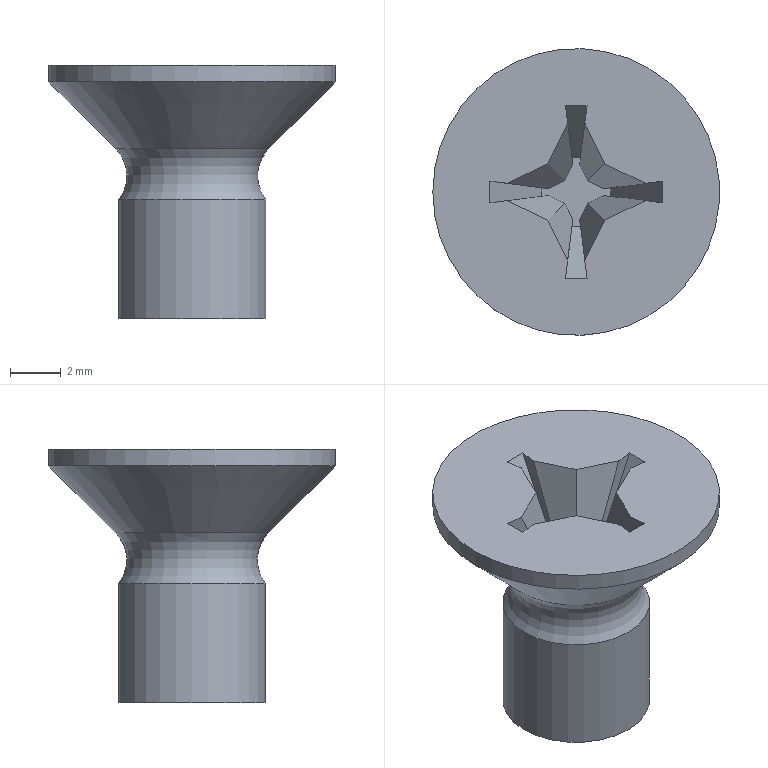Part | NX | features SKETCH 3, DATUM_CSYS 2, DATUM_PLANE 1, FSET 1, LINE 1, META 1, SKIN 1, SWP104 1, SYMBOLIC_THREAD 1, THREADS 1 | 1 solid | 27 faces | box 11.3 x 11.3 x 10 mm | volume 366.572 mm3 | plane 23 | cylinder 2 | torus 1 | cone 1 | commonest cylinder face diameters 5.795 x1 11.3 x1
STEP:
#1=CARTESIAN_POINT('',(-2.897,0.,-5.3));
#2=VERTEX_POINT('',#1);
#3=CARTESIAN_POINT('',(0.,0.,-5.3));
#4=DIRECTION('',(0.,0.,-1.));
#5=DIRECTION('',(-1.,0.,0.));
#6=AXIS2_PLACEMENT_3D('',#3,#4,#5);
#7=CIRCLE('',#6,2.897);
#8=EDGE_CURVE('',#2,#2,#7,.T.);
#9=ORIENTED_EDGE('',*,*,#8,.F.);
#10=EDGE_LOOP('',(#9));
#11=FACE_BOUND('',#10,.T.);
#12=CARTESIAN_POINT('',(-3.014,0.,-3.3));
#13=VERTEX_POINT('',#12);
#14=CARTESIAN_POINT('',(0.,0.,-3.3));
#15=DIRECTION('',(0.,0.,-1.));
#16=DIRECTION('',(-1.,0.,0.));
#17=AXIS2_PLACEMENT_3D('',#14,#15,#16);
#18=CIRCLE('',#17,3.014);
#19=EDGE_CURVE('',#13,#13,#18,.T.);
#20=ORIENTED_EDGE('',*,*,#19,.T.);
#21=EDGE_LOOP('',(#20));
#22=FACE_BOUND('',#21,.T.);
#23=CARTESIAN_POINT('',(0.,0.,-4.366));
#24=DIRECTION('',(0.,0.,-1.));
#25=DIRECTION('',(-1.,0.,0.));
#26=AXIS2_PLACEMENT_3D('',#23,#24,#25);
#27=TOROIDAL_SURFACE('',#26,4.08,1.507);
#28=ADVANCED_FACE('',(#11,#22),#27,.F.);
#29=CARTESIAN_POINT('',(-2.898,0.,-10.));
#30=VERTEX_POINT('',#29);
#31=CARTESIAN_POINT('',(0.,0.,-10.));
#32=DIRECTION('',(0.,0.,-1.));
#33=DIRECTION('',(-1.,0.,0.));
#34=AXIS2_PLACEMENT_3D('',#31,#32,#33);
#35=CIRCLE('',#34,2.898);
#36=EDGE_CURVE('',#30,#30,#35,.T.);
#37=ORIENTED_EDGE('',*,*,#36,.F.);
#38=EDGE_LOOP('',(#37));
#39=FACE_BOUND('',#38,.T.);
#40=ORIENTED_EDGE('',*,*,#8,.T.);
#41=EDGE_LOOP('',(#40));
#42=FACE_BOUND('',#41,.T.);
#43=CARTESIAN_POINT('',(0.,0.,0.));
#44=DIRECTION('',(0.,0.,-1.));
#45=DIRECTION('',(-1.,0.,0.));
#46=AXIS2_PLACEMENT_3D('',#43,#44,#45);
#47=CYLINDRICAL_SURFACE('',#46,2.898);
#48=ADVANCED_FACE('',(#39,#42),#47,.T.);
#49=ORIENTED_EDGE('',*,*,#36,.T.);
#50=EDGE_LOOP('',(#49));
#51=FACE_BOUND('',#50,.T.);
#52=CARTESIAN_POINT('',(0.,2.898,-10.));
#53=DIRECTION('',(0.,0.,1.));
#54=DIRECTION('',(1.,0.,0.));
#55=AXIS2_PLACEMENT_3D('',#52,#53,#54);
#56=PLANE('',#55);
#57=ADVANCED_FACE('',(#51),#56,.F.);
#58=CARTESIAN_POINT('',(3.4,-0.425,0.));
#59=VERTEX_POINT('',#58);
#60=CARTESIAN_POINT('',(2.72,-0.34,0.));
#61=VERTEX_POINT('',#60);
#62=CARTESIAN_POINT('',(3.06,-0.3825,0.));
#63=DIRECTION('',(-0.9923,0.124,0.));
#64=VECTOR('',#63,1000.);
#65=LINE('',#62,#64);
#66=EDGE_CURVE('',#59,#61,#65,.T.);
#67=ORIENTED_EDGE('',*,*,#66,.T.);
#68=CARTESIAN_POINT('',(1.117,-1.117,0.));
#69=VERTEX_POINT('',#68);
#70=CARTESIAN_POINT('',(1.919,-0.7287,0.));
#71=DIRECTION('',(-0.8997,-0.4364,0.));
#72=VECTOR('',#71,1000.);
#73=LINE('',#70,#72);
#74=EDGE_CURVE('',#61,#69,#73,.T.);
#75=ORIENTED_EDGE('',*,*,#74,.T.);
#76=CARTESIAN_POINT('',(0.34,-2.72,0.));
#77=VERTEX_POINT('',#76);
#78=CARTESIAN_POINT('',(0.7287,-1.919,0.));
#79=DIRECTION('',(-0.4364,-0.8997,0.));
#80=VECTOR('',#79,1000.);
#81=LINE('',#78,#80);
#82=EDGE_CURVE('',#69,#77,#81,.T.);
#83=ORIENTED_EDGE('',*,*,#82,.T.);
#84=CARTESIAN_POINT('',(0.425,-3.4,0.));
#85=VERTEX_POINT('',#84);
#86=CARTESIAN_POINT('',(0.3825,-3.06,0.));
#87=DIRECTION('',(0.124,-0.9923,0.));
#88=VECTOR('',#87,1000.);
#89=LINE('',#86,#88);
#90=EDGE_CURVE('',#77,#85,#89,.T.);
#91=ORIENTED_EDGE('',*,*,#90,.T.);
#92=CARTESIAN_POINT('',(-0.425,-3.4,0.));
#93=VERTEX_POINT('',#92);
#94=CARTESIAN_POINT('',(0.2125,-3.4,0.));
#95=DIRECTION('',(-1.,0.,0.));
#96=VECTOR('',#95,1000.);
#97=LINE('',#94,#96);
#98=EDGE_CURVE('',#85,#93,#97,.T.);
#99=ORIENTED_EDGE('',*,*,#98,.T.);
#100=CARTESIAN_POINT('',(-0.34,-2.72,0.));
#101=VERTEX_POINT('',#100);
#102=CARTESIAN_POINT('',(-0.3825,-3.06,0.));
#103=DIRECTION('',(0.124,0.9923,0.));
#104=VECTOR('',#103,1000.);
#105=LINE('',#102,#104);
#106=EDGE_CURVE('',#93,#101,#105,.T.);
#107=ORIENTED_EDGE('',*,*,#106,.T.);
#108=CARTESIAN_POINT('',(-1.117,-1.117,0.));
#109=VERTEX_POINT('',#108);
#110=CARTESIAN_POINT('',(-0.7287,-1.919,0.));
#111=DIRECTION('',(-0.4364,0.8997,0.));
#112=VECTOR('',#111,1000.);
#113=LINE('',#110,#112);
#114=EDGE_CURVE('',#101,#109,#113,.T.);
#115=ORIENTED_EDGE('',*,*,#114,.T.);
#116=CARTESIAN_POINT('',(-2.72,-0.34,0.));
#117=VERTEX_POINT('',#116);
#118=CARTESIAN_POINT('',(-1.919,-0.7287,0.));
#119=DIRECTION('',(-0.8997,0.4364,0.));
#120=VECTOR('',#119,1000.);
#121=LINE('',#118,#120);
#122=EDGE_CURVE('',#109,#117,#121,.T.);
#123=ORIENTED_EDGE('',*,*,#122,.T.);
#124=CARTESIAN_POINT('',(-3.4,-0.425,0.));
#125=VERTEX_POINT('',#124);
#126=CARTESIAN_POINT('',(-3.06,-0.3825,0.));
#127=DIRECTION('',(-0.9923,-0.124,0.));
#128=VECTOR('',#127,1000.);
#129=LINE('',#126,#128);
#130=EDGE_CURVE('',#117,#125,#129,.T.);
#131=ORIENTED_EDGE('',*,*,#130,.T.);
#132=CARTESIAN_POINT('',(-3.4,0.425,0.));
#133=VERTEX_POINT('',#132);
#134=CARTESIAN_POINT('',(-3.4,-0.2125,0.));
#135=DIRECTION('',(0.,1.,0.));
#136=VECTOR('',#135,1000.);
#137=LINE('',#134,#136);
#138=EDGE_CURVE('',#125,#133,#137,.T.);
#139=ORIENTED_EDGE('',*,*,#138,.T.);
#140=CARTESIAN_POINT('',(-2.72,0.34,0.));
#141=VERTEX_POINT('',#140);
#142=CARTESIAN_POINT('',(-3.06,0.3825,0.));
#143=DIRECTION('',(0.9923,-0.124,0.));
#144=VECTOR('',#143,1000.);
#145=LINE('',#142,#144);
#146=EDGE_CURVE('',#133,#141,#145,.T.);
#147=ORIENTED_EDGE('',*,*,#146,.T.);
#148=CARTESIAN_POINT('',(-1.117,1.117,0.));
#149=VERTEX_POINT('',#148);
#150=CARTESIAN_POINT('',(-1.919,0.7287,0.));
#151=DIRECTION('',(0.8997,0.4364,0.));
#152=VECTOR('',#151,1000.);
#153=LINE('',#150,#152);
#154=EDGE_CURVE('',#141,#149,#153,.T.);
#155=ORIENTED_EDGE('',*,*,#154,.T.);
#156=CARTESIAN_POINT('',(-0.34,2.72,0.));
#157=VERTEX_POINT('',#156);
#158=CARTESIAN_POINT('',(-0.7287,1.919,0.));
#159=DIRECTION('',(0.4364,0.8997,0.));
#160=VECTOR('',#159,1000.);
#161=LINE('',#158,#160);
#162=EDGE_CURVE('',#149,#157,#161,.T.);
#163=ORIENTED_EDGE('',*,*,#162,.T.);
#164=CARTESIAN_POINT('',(-0.425,3.4,0.));
#165=VERTEX_POINT('',#164);
#166=CARTESIAN_POINT('',(-0.3825,3.06,0.));
#167=DIRECTION('',(-0.124,0.9923,0.));
#168=VECTOR('',#167,1000.);
#169=LINE('',#166,#168);
#170=EDGE_CURVE('',#157,#165,#169,.T.);
#171=ORIENTED_EDGE('',*,*,#170,.T.);
#172=CARTESIAN_POINT('',(0.425,3.4,0.));
#173=VERTEX_POINT('',#172);
#174=CARTESIAN_POINT('',(-0.2125,3.4,0.));
#175=DIRECTION('',(1.,0.,0.));
#176=VECTOR('',#175,1000.);
#177=LINE('',#174,#176);
#178=EDGE_CURVE('',#165,#173,#177,.T.);
#179=ORIENTED_EDGE('',*,*,#178,.T.);
#180=CARTESIAN_POINT('',(0.34,2.72,0.));
#181=VERTEX_POINT('',#180);
#182=CARTESIAN_POINT('',(0.3825,3.06,0.));
#183=DIRECTION('',(-0.124,-0.9923,0.));
#184=VECTOR('',#183,1000.);
#185=LINE('',#182,#184);
#186=EDGE_CURVE('',#173,#181,#185,.T.);
#187=ORIENTED_EDGE('',*,*,#186,.T.);
#188=CARTESIAN_POINT('',(1.117,1.117,0.));
#189=VERTEX_POINT('',#188);
#190=CARTESIAN_POINT('',(0.7287,1.919,0.));
#191=DIRECTION('',(0.4364,-0.8997,0.));
#192=VECTOR('',#191,1000.);
#193=LINE('',#190,#192);
#194=EDGE_CURVE('',#181,#189,#193,.T.);
#195=ORIENTED_EDGE('',*,*,#194,.T.);
#196=CARTESIAN_POINT('',(2.72,0.34,0.));
#197=VERTEX_POINT('',#196);
#198=CARTESIAN_POINT('',(1.919,0.7287,0.));
#199=DIRECTION('',(0.8997,-0.4364,0.));
#200=VECTOR('',#199,1000.);
#201=LINE('',#198,#200);
#202=EDGE_CURVE('',#189,#197,#201,.T.);
#203=ORIENTED_EDGE('',*,*,#202,.T.);
#204=CARTESIAN_POINT('',(3.4,0.425,0.));
#205=VERTEX_POINT('',#204);
#206=CARTESIAN_POINT('',(3.06,0.3825,0.));
#207=DIRECTION('',(0.9923,0.124,0.));
#208=VECTOR('',#207,1000.);
#209=LINE('',#206,#208);
#210=EDGE_CURVE('',#197,#205,#209,.T.);
#211=ORIENTED_EDGE('',*,*,#210,.T.);
#212=CARTESIAN_POINT('',(3.4,0.2125,0.));
#213=DIRECTION('',(0.,-1.,0.));
#214=VECTOR('',#213,1000.);
#215=LINE('',#212,#214);
#216=EDGE_CURVE('',#205,#59,#215,.T.);
#217=ORIENTED_EDGE('',*,*,#216,.T.);
#218=EDGE_LOOP('',(#67,#75,#83,#91,#99,#107,#115,#123,#131,#139,#147,#155,#163,#171,#179,#187,#195,#203,#211,#217));
#219=FACE_BOUND('',#218,.T.);
#220=CARTESIAN_POINT('',(-5.65,0.,0.));
#221=VERTEX_POINT('',#220);
#222=CARTESIAN_POINT('',(0.,0.,0.));
#223=DIRECTION('',(0.,0.,-1.));
#224=DIRECTION('',(-1.,0.,0.));
#225=AXIS2_PLACEMENT_3D('',#222,#223,#224);
#226=CIRCLE('',#225,5.65);
#227=EDGE_CURVE('',#221,#221,#226,.T.);
#228=ORIENTED_EDGE('',*,*,#227,.F.);
#229=EDGE_LOOP('',(#228));
#230=FACE_BOUND('',#229,.T.);
#231=CARTESIAN_POINT('',(0.,0.,0.));
#232=DIRECTION('',(0.,0.,-1.));
#233=DIRECTION('',(-1.,0.,0.));
#234=AXIS2_PLACEMENT_3D('',#231,#232,#233);
#235=PLANE('',#234);
#236=ADVANCED_FACE('',(#219,#230),#235,.F.);
#237=CARTESIAN_POINT('',(-5.65,0.,-0.6641));
#238=VERTEX_POINT('',#237);
#239=CARTESIAN_POINT('',(0.,0.,-0.6641));
#240=DIRECTION('',(0.,0.,-1.));
#241=DIRECTION('',(-1.,0.,0.));
#242=AXIS2_PLACEMENT_3D('',#239,#240,#241);
#243=CIRCLE('',#242,5.65);
#244=EDGE_CURVE('',#238,#238,#243,.T.);
#245=ORIENTED_EDGE('',*,*,#244,.F.);
#246=EDGE_LOOP('',(#245));
#247=FACE_BOUND('',#246,.T.);
#248=ORIENTED_EDGE('',*,*,#227,.T.);
#249=EDGE_LOOP('',(#248));
#250=FACE_BOUND('',#249,.T.);
#251=CARTESIAN_POINT('',(0.,0.,0.));
#252=DIRECTION('',(0.,0.,-1.));
#253=DIRECTION('',(-1.,0.,0.));
#254=AXIS2_PLACEMENT_3D('',#251,#252,#253);
#255=CYLINDRICAL_SURFACE('',#254,5.65);
#256=ADVANCED_FACE('',(#247,#250),#255,.T.);
#257=ORIENTED_EDGE('',*,*,#19,.F.);
#258=EDGE_LOOP('',(#257));
#259=FACE_BOUND('',#258,.T.);
#260=ORIENTED_EDGE('',*,*,#244,.T.);
#261=EDGE_LOOP('',(#260));
#262=FACE_BOUND('',#261,.T.);
#263=CARTESIAN_POINT('',(0.,0.,-0.6641));
#264=DIRECTION('',(0.,0.,1.));
#265=DIRECTION('',(1.,0.,0.));
#266=AXIS2_PLACEMENT_3D('',#263,#264,#265);
#267=CONICAL_SURFACE('',#266,5.65,0.7854);
#268=ADVANCED_FACE('',(#259,#262),#267,.T.);
#269=CARTESIAN_POINT('',(1.36,-0.17,-3.5));
#270=VERTEX_POINT('',#269);
#271=CARTESIAN_POINT('',(2.38,-0.2975,-1.75));
#272=DIRECTION('',(0.5026,-0.06282,0.8623));
#273=VECTOR('',#272,1000.);
#274=LINE('',#271,#273);
#275=EDGE_CURVE('',#270,#59,#274,.T.);
#276=ORIENTED_EDGE('',*,*,#275,.F.);
#277=CARTESIAN_POINT('',(1.088,-0.136,-3.5));
#278=VERTEX_POINT('',#277);
#279=CARTESIAN_POINT('',(1.224,-0.153,-3.5));
#280=DIRECTION('',(-0.9923,0.124,0.));
#281=VECTOR('',#280,1000.);
#282=LINE('',#279,#281);
#283=EDGE_CURVE('',#270,#278,#282,.T.);
#284=ORIENTED_EDGE('',*,*,#283,.T.);
#285=CARTESIAN_POINT('',(1.904,-0.238,-1.75));
#286=DIRECTION('',(0.422,-0.05275,0.9051));
#287=VECTOR('',#286,1000.);
#288=LINE('',#285,#287);
#289=EDGE_CURVE('',#278,#61,#288,.T.);
#290=ORIENTED_EDGE('',*,*,#289,.T.);
#291=ORIENTED_EDGE('',*,*,#66,.F.);
#292=EDGE_LOOP('',(#276,#284,#290,#291));
#293=FACE_BOUND('',#292,.T.);
#294=CARTESIAN_POINT('',(2.38,-0.2975,-1.75));
#295=DIRECTION('',(0.124,0.9923,0.));
#296=DIRECTION('',(-0.9923,0.124,0.));
#297=AXIS2_PLACEMENT_3D('',#294,#295,#296);
#298=PLANE('',#297);
#299=ADVANCED_FACE('',(#293),#298,.T.);
#300=CARTESIAN_POINT('',(1.36,0.17,-3.5));
#301=VERTEX_POINT('',#300);
#302=CARTESIAN_POINT('',(2.38,0.2975,-1.75));
#303=DIRECTION('',(0.5026,0.06282,0.8623));
#304=VECTOR('',#303,1000.);
#305=LINE('',#302,#304);
#306=EDGE_CURVE('',#301,#205,#305,.T.);
#307=ORIENTED_EDGE('',*,*,#306,.F.);
#308=CARTESIAN_POINT('',(1.36,0.085,-3.5));
#309=DIRECTION('',(0.,-1.,0.));
#310=VECTOR('',#309,1000.);
#311=LINE('',#308,#310);
#312=EDGE_CURVE('',#301,#270,#311,.T.);
#313=ORIENTED_EDGE('',*,*,#312,.T.);
#314=ORIENTED_EDGE('',*,*,#275,.T.);
#315=ORIENTED_EDGE('',*,*,#216,.F.);
#316=EDGE_LOOP('',(#307,#313,#314,#315));
#317=FACE_BOUND('',#316,.T.);
#318=CARTESIAN_POINT('',(2.38,0.2975,-1.75));
#319=DIRECTION('',(-0.864,0.,0.5036));
#320=DIRECTION('',(0.5036,0.,0.864));
#321=AXIS2_PLACEMENT_3D('',#318,#319,#320);
#322=PLANE('',#321);
#323=ADVANCED_FACE('',(#317),#322,.T.);
#324=CARTESIAN_POINT('',(1.088,0.136,-3.5));
#325=VERTEX_POINT('',#324);
#326=CARTESIAN_POINT('',(1.904,0.238,-1.75));
#327=DIRECTION('',(0.422,0.05275,0.9051));
#328=VECTOR('',#327,1000.);
#329=LINE('',#326,#328);
#330=EDGE_CURVE('',#325,#197,#329,.T.);
#331=ORIENTED_EDGE('',*,*,#330,.F.);
#332=CARTESIAN_POINT('',(1.224,0.153,-3.5));
#333=DIRECTION('',(0.9923,0.124,0.));
#334=VECTOR('',#333,1000.);
#335=LINE('',#332,#334);
#336=EDGE_CURVE('',#325,#301,#335,.T.);
#337=ORIENTED_EDGE('',*,*,#336,.T.);
#338=ORIENTED_EDGE('',*,*,#306,.T.);
#339=ORIENTED_EDGE('',*,*,#210,.F.);
#340=EDGE_LOOP('',(#331,#337,#338,#339));
#341=FACE_BOUND('',#340,.T.);
#342=CARTESIAN_POINT('',(2.38,0.2975,-1.75));
#343=DIRECTION('',(0.124,-0.9923,0.));
#344=DIRECTION('',(0.9923,0.124,0.));
#345=AXIS2_PLACEMENT_3D('',#342,#343,#344);
#346=PLANE('',#345);
#347=ADVANCED_FACE('',(#341),#346,.T.);
#348=CARTESIAN_POINT('',(0.4469,0.4469,-3.5));
#349=VERTEX_POINT('',#348);
#350=CARTESIAN_POINT('',(0.7821,0.7821,-1.75));
#351=DIRECTION('',(0.1849,0.1849,0.9652));
#352=VECTOR('',#351,1000.);
#353=LINE('',#350,#352);
#354=EDGE_CURVE('',#349,#189,#353,.T.);
#355=ORIENTED_EDGE('',*,*,#354,.F.);
#356=CARTESIAN_POINT('',(0.7675,0.2915,-3.5));
#357=DIRECTION('',(0.8997,-0.4364,0.));
#358=VECTOR('',#357,1000.);
#359=LINE('',#356,#358);
#360=EDGE_CURVE('',#349,#325,#359,.T.);
#361=ORIENTED_EDGE('',*,*,#360,.T.);
#362=ORIENTED_EDGE('',*,*,#330,.T.);
#363=ORIENTED_EDGE('',*,*,#202,.F.);
#364=EDGE_LOOP('',(#355,#361,#362,#363));
#365=FACE_BOUND('',#364,.T.);
#366=CARTESIAN_POINT('',(1.904,0.238,-1.75));
#367=DIRECTION('',(-0.4228,-0.8717,0.2479));
#368=DIRECTION('',(0.8997,-0.4364,0.));
#369=AXIS2_PLACEMENT_3D('',#366,#367,#368);
#370=PLANE('',#369);
#371=ADVANCED_FACE('',(#365),#370,.T.);
#372=CARTESIAN_POINT('',(0.136,1.088,-3.5));
#373=VERTEX_POINT('',#372);
#374=CARTESIAN_POINT('',(0.238,1.904,-1.75));
#375=DIRECTION('',(0.05275,0.422,0.9051));
#376=VECTOR('',#375,1000.);
#377=LINE('',#374,#376);
#378=EDGE_CURVE('',#373,#181,#377,.T.);
#379=ORIENTED_EDGE('',*,*,#378,.F.);
#380=CARTESIAN_POINT('',(0.2915,0.7675,-3.5));
#381=DIRECTION('',(0.4364,-0.8997,0.));
#382=VECTOR('',#381,1000.);
#383=LINE('',#380,#382);
#384=EDGE_CURVE('',#373,#349,#383,.T.);
#385=ORIENTED_EDGE('',*,*,#384,.T.);
#386=ORIENTED_EDGE('',*,*,#354,.T.);
#387=ORIENTED_EDGE('',*,*,#194,.F.);
#388=EDGE_LOOP('',(#379,#385,#386,#387));
#389=FACE_BOUND('',#388,.T.);
#390=CARTESIAN_POINT('',(0.238,1.904,-1.75));
#391=DIRECTION('',(-0.8717,-0.4228,0.2479));
#392=DIRECTION('',(0.4364,-0.8997,0.));
#393=AXIS2_PLACEMENT_3D('',#390,#391,#392);
#394=PLANE('',#393);
#395=ADVANCED_FACE('',(#389),#394,.T.);
#396=CARTESIAN_POINT('',(0.17,1.36,-3.5));
#397=VERTEX_POINT('',#396);
#398=CARTESIAN_POINT('',(0.2975,2.38,-1.75));
#399=DIRECTION('',(0.06282,0.5026,0.8623));
#400=VECTOR('',#399,1000.);
#401=LINE('',#398,#400);
#402=EDGE_CURVE('',#397,#173,#401,.T.);
#403=ORIENTED_EDGE('',*,*,#402,.F.);
#404=CARTESIAN_POINT('',(0.153,1.224,-3.5));
#405=DIRECTION('',(-0.124,-0.9923,0.));
#406=VECTOR('',#405,1000.);
#407=LINE('',#404,#406);
#408=EDGE_CURVE('',#397,#373,#407,.T.);
#409=ORIENTED_EDGE('',*,*,#408,.T.);
#410=ORIENTED_EDGE('',*,*,#378,.T.);
#411=ORIENTED_EDGE('',*,*,#186,.F.);
#412=EDGE_LOOP('',(#403,#409,#410,#411));
#413=FACE_BOUND('',#412,.T.);
#414=CARTESIAN_POINT('',(0.2975,2.38,-1.75));
#415=DIRECTION('',(-0.9923,0.124,0.));
#416=DIRECTION('',(-0.124,-0.9923,0.));
#417=AXIS2_PLACEMENT_3D('',#414,#415,#416);
#418=PLANE('',#417);
#419=ADVANCED_FACE('',(#413),#418,.T.);
#420=CARTESIAN_POINT('',(-0.17,1.36,-3.5));
#421=VERTEX_POINT('',#420);
#422=CARTESIAN_POINT('',(-0.2975,2.38,-1.75));
#423=DIRECTION('',(-0.06282,0.5026,0.8623));
#424=VECTOR('',#423,1000.);
#425=LINE('',#422,#424);
#426=EDGE_CURVE('',#421,#165,#425,.T.);
#427=ORIENTED_EDGE('',*,*,#426,.F.);
#428=CARTESIAN_POINT('',(-0.085,1.36,-3.5));
#429=DIRECTION('',(1.,0.,0.));
#430=VECTOR('',#429,1000.);
#431=LINE('',#428,#430);
#432=EDGE_CURVE('',#421,#397,#431,.T.);
#433=ORIENTED_EDGE('',*,*,#432,.T.);
#434=ORIENTED_EDGE('',*,*,#402,.T.);
#435=ORIENTED_EDGE('',*,*,#178,.F.);
#436=EDGE_LOOP('',(#427,#433,#434,#435));
#437=FACE_BOUND('',#436,.T.);
#438=CARTESIAN_POINT('',(-0.2975,2.38,-1.75));
#439=DIRECTION('',(0.,-0.864,0.5036));
#440=DIRECTION('',(0.,-0.5036,-0.864));
#441=AXIS2_PLACEMENT_3D('',#438,#439,#440);
#442=PLANE('',#441);
#443=ADVANCED_FACE('',(#437),#442,.T.);
#444=CARTESIAN_POINT('',(-0.136,1.088,-3.5));
#445=VERTEX_POINT('',#444);
#446=CARTESIAN_POINT('',(-0.238,1.904,-1.75));
#447=DIRECTION('',(-0.05275,0.422,0.9051));
#448=VECTOR('',#447,1000.);
#449=LINE('',#446,#448);
#450=EDGE_CURVE('',#445,#157,#449,.T.);
#451=ORIENTED_EDGE('',*,*,#450,.F.);
#452=CARTESIAN_POINT('',(-0.153,1.224,-3.5));
#453=DIRECTION('',(-0.124,0.9923,0.));
#454=VECTOR('',#453,1000.);
#455=LINE('',#452,#454);
#456=EDGE_CURVE('',#445,#421,#455,.T.);
#457=ORIENTED_EDGE('',*,*,#456,.T.);
#458=ORIENTED_EDGE('',*,*,#426,.T.);
#459=ORIENTED_EDGE('',*,*,#170,.F.);
#460=EDGE_LOOP('',(#451,#457,#458,#459));
#461=FACE_BOUND('',#460,.T.);
#462=CARTESIAN_POINT('',(-0.2975,2.38,-1.75));
#463=DIRECTION('',(0.9923,0.124,0.));
#464=DIRECTION('',(-0.124,0.9923,0.));
#465=AXIS2_PLACEMENT_3D('',#462,#463,#464);
#466=PLANE('',#465);
#467=ADVANCED_FACE('',(#461),#466,.T.);
#468=CARTESIAN_POINT('',(-0.4469,0.4469,-3.5));
#469=VERTEX_POINT('',#468);
#470=CARTESIAN_POINT('',(-0.7821,0.7821,-1.75));
#471=DIRECTION('',(-0.1849,0.1849,0.9652));
#472=VECTOR('',#471,1000.);
#473=LINE('',#470,#472);
#474=EDGE_CURVE('',#469,#149,#473,.T.);
#475=ORIENTED_EDGE('',*,*,#474,.F.);
#476=CARTESIAN_POINT('',(-0.2915,0.7675,-3.5));
#477=DIRECTION('',(0.4364,0.8997,0.));
#478=VECTOR('',#477,1000.);
#479=LINE('',#476,#478);
#480=EDGE_CURVE('',#469,#445,#479,.T.);
#481=ORIENTED_EDGE('',*,*,#480,.T.);
#482=ORIENTED_EDGE('',*,*,#450,.T.);
#483=ORIENTED_EDGE('',*,*,#162,.F.);
#484=EDGE_LOOP('',(#475,#481,#482,#483));
#485=FACE_BOUND('',#484,.T.);
#486=CARTESIAN_POINT('',(-0.238,1.904,-1.75));
#487=DIRECTION('',(0.8717,-0.4228,0.2479));
#488=DIRECTION('',(0.4364,0.8997,0.));
#489=AXIS2_PLACEMENT_3D('',#486,#487,#488);
#490=PLANE('',#489);
#491=ADVANCED_FACE('',(#485),#490,.T.);
#492=CARTESIAN_POINT('',(-1.088,0.136,-3.5));
#493=VERTEX_POINT('',#492);
#494=CARTESIAN_POINT('',(-1.904,0.238,-1.75));
#495=DIRECTION('',(-0.422,0.05275,0.9051));
#496=VECTOR('',#495,1000.);
#497=LINE('',#494,#496);
#498=EDGE_CURVE('',#493,#141,#497,.T.);
#499=ORIENTED_EDGE('',*,*,#498,.F.);
#500=CARTESIAN_POINT('',(-0.7675,0.2915,-3.5));
#501=DIRECTION('',(0.8997,0.4364,0.));
#502=VECTOR('',#501,1000.);
#503=LINE('',#500,#502);
#504=EDGE_CURVE('',#493,#469,#503,.T.);
#505=ORIENTED_EDGE('',*,*,#504,.T.);
#506=ORIENTED_EDGE('',*,*,#474,.T.);
#507=ORIENTED_EDGE('',*,*,#154,.F.);
#508=EDGE_LOOP('',(#499,#505,#506,#507));
#509=FACE_BOUND('',#508,.T.);
#510=CARTESIAN_POINT('',(-1.904,0.238,-1.75));
#511=DIRECTION('',(0.4228,-0.8717,0.2479));
#512=DIRECTION('',(0.8997,0.4364,0.));
#513=AXIS2_PLACEMENT_3D('',#510,#511,#512);
#514=PLANE('',#513);
#515=ADVANCED_FACE('',(#509),#514,.T.);
#516=CARTESIAN_POINT('',(-1.36,0.17,-3.5));
#517=VERTEX_POINT('',#516);
#518=CARTESIAN_POINT('',(-2.38,0.2975,-1.75));
#519=DIRECTION('',(-0.5026,0.06282,0.8623));
#520=VECTOR('',#519,1000.);
#521=LINE('',#518,#520);
#522=EDGE_CURVE('',#517,#133,#521,.T.);
#523=ORIENTED_EDGE('',*,*,#522,.F.);
#524=CARTESIAN_POINT('',(-1.224,0.153,-3.5));
#525=DIRECTION('',(0.9923,-0.124,0.));
#526=VECTOR('',#525,1000.);
#527=LINE('',#524,#526);
#528=EDGE_CURVE('',#517,#493,#527,.T.);
#529=ORIENTED_EDGE('',*,*,#528,.T.);
#530=ORIENTED_EDGE('',*,*,#498,.T.);
#531=ORIENTED_EDGE('',*,*,#146,.F.);
#532=EDGE_LOOP('',(#523,#529,#530,#531));
#533=FACE_BOUND('',#532,.T.);
#534=CARTESIAN_POINT('',(-2.38,0.2975,-1.75));
#535=DIRECTION('',(-0.124,-0.9923,0.));
#536=DIRECTION('',(0.9923,-0.124,0.));
#537=AXIS2_PLACEMENT_3D('',#534,#535,#536);
#538=PLANE('',#537);
#539=ADVANCED_FACE('',(#533),#538,.T.);
#540=CARTESIAN_POINT('',(-1.36,-0.17,-3.5));
#541=VERTEX_POINT('',#540);
#542=CARTESIAN_POINT('',(-2.38,-0.2975,-1.75));
#543=DIRECTION('',(-0.5026,-0.06282,0.8623));
#544=VECTOR('',#543,1000.);
#545=LINE('',#542,#544);
#546=EDGE_CURVE('',#541,#125,#545,.T.);
#547=ORIENTED_EDGE('',*,*,#546,.F.);
#548=CARTESIAN_POINT('',(-1.36,-0.085,-3.5));
#549=DIRECTION('',(0.,1.,0.));
#550=VECTOR('',#549,1000.);
#551=LINE('',#548,#550);
#552=EDGE_CURVE('',#541,#517,#551,.T.);
#553=ORIENTED_EDGE('',*,*,#552,.T.);
#554=ORIENTED_EDGE('',*,*,#522,.T.);
#555=ORIENTED_EDGE('',*,*,#138,.F.);
#556=EDGE_LOOP('',(#547,#553,#554,#555));
#557=FACE_BOUND('',#556,.T.);
#558=CARTESIAN_POINT('',(-2.38,-0.2975,-1.75));
#559=DIRECTION('',(0.864,0.,0.5036));
#560=DIRECTION('',(0.5036,0.,-0.864));
#561=AXIS2_PLACEMENT_3D('',#558,#559,#560);
#562=PLANE('',#561);
#563=ADVANCED_FACE('',(#557),#562,.T.);
#564=CARTESIAN_POINT('',(-1.088,-0.136,-3.5));
#565=VERTEX_POINT('',#564);
#566=CARTESIAN_POINT('',(-1.904,-0.238,-1.75));
#567=DIRECTION('',(-0.422,-0.05275,0.9051));
#568=VECTOR('',#567,1000.);
#569=LINE('',#566,#568);
#570=EDGE_CURVE('',#565,#117,#569,.T.);
#571=ORIENTED_EDGE('',*,*,#570,.F.);
#572=CARTESIAN_POINT('',(-1.224,-0.153,-3.5));
#573=DIRECTION('',(-0.9923,-0.124,0.));
#574=VECTOR('',#573,1000.);
#575=LINE('',#572,#574);
#576=EDGE_CURVE('',#565,#541,#575,.T.);
#577=ORIENTED_EDGE('',*,*,#576,.T.);
#578=ORIENTED_EDGE('',*,*,#546,.T.);
#579=ORIENTED_EDGE('',*,*,#130,.F.);
#580=EDGE_LOOP('',(#571,#577,#578,#579));
#581=FACE_BOUND('',#580,.T.);
#582=CARTESIAN_POINT('',(-2.38,-0.2975,-1.75));
#583=DIRECTION('',(-0.124,0.9923,0.));
#584=DIRECTION('',(-0.9923,-0.124,0.));
#585=AXIS2_PLACEMENT_3D('',#582,#583,#584);
#586=PLANE('',#585);
#587=ADVANCED_FACE('',(#581),#586,.T.);
#588=CARTESIAN_POINT('',(-0.4469,-0.4469,-3.5));
#589=VERTEX_POINT('',#588);
#590=CARTESIAN_POINT('',(-0.7821,-0.7821,-1.75));
#591=DIRECTION('',(-0.1849,-0.1849,0.9652));
#592=VECTOR('',#591,1000.);
#593=LINE('',#590,#592);
#594=EDGE_CURVE('',#589,#109,#593,.T.);
#595=ORIENTED_EDGE('',*,*,#594,.F.);
#596=CARTESIAN_POINT('',(-0.7675,-0.2915,-3.5));
#597=DIRECTION('',(-0.8997,0.4364,0.));
#598=VECTOR('',#597,1000.);
#599=LINE('',#596,#598);
#600=EDGE_CURVE('',#589,#565,#599,.T.);
#601=ORIENTED_EDGE('',*,*,#600,.T.);
#602=ORIENTED_EDGE('',*,*,#570,.T.);
#603=ORIENTED_EDGE('',*,*,#122,.F.);
#604=EDGE_LOOP('',(#595,#601,#602,#603));
#605=FACE_BOUND('',#604,.T.);
#606=CARTESIAN_POINT('',(-1.904,-0.238,-1.75));
#607=DIRECTION('',(0.4228,0.8717,0.2479));
#608=DIRECTION('',(-0.8997,0.4364,0.));
#609=AXIS2_PLACEMENT_3D('',#606,#607,#608);
#610=PLANE('',#609);
#611=ADVANCED_FACE('',(#605),#610,.T.);
#612=CARTESIAN_POINT('',(-0.136,-1.088,-3.5));
#613=VERTEX_POINT('',#612);
#614=CARTESIAN_POINT('',(-0.238,-1.904,-1.75));
#615=DIRECTION('',(-0.05275,-0.422,0.9051));
#616=VECTOR('',#615,1000.);
#617=LINE('',#614,#616);
#618=EDGE_CURVE('',#613,#101,#617,.T.);
#619=ORIENTED_EDGE('',*,*,#618,.F.);
#620=CARTESIAN_POINT('',(-0.2915,-0.7675,-3.5));
#621=DIRECTION('',(-0.4364,0.8997,0.));
#622=VECTOR('',#621,1000.);
#623=LINE('',#620,#622);
#624=EDGE_CURVE('',#613,#589,#623,.T.);
#625=ORIENTED_EDGE('',*,*,#624,.T.);
#626=ORIENTED_EDGE('',*,*,#594,.T.);
#627=ORIENTED_EDGE('',*,*,#114,.F.);
#628=EDGE_LOOP('',(#619,#625,#626,#627));
#629=FACE_BOUND('',#628,.T.);
#630=CARTESIAN_POINT('',(-0.238,-1.904,-1.75));
#631=DIRECTION('',(0.8717,0.4228,0.2479));
#632=DIRECTION('',(-0.4364,0.8997,0.));
#633=AXIS2_PLACEMENT_3D('',#630,#631,#632);
#634=PLANE('',#633);
#635=ADVANCED_FACE('',(#629),#634,.T.);
#636=CARTESIAN_POINT('',(-0.17,-1.36,-3.5));
#637=VERTEX_POINT('',#636);
#638=CARTESIAN_POINT('',(-0.2975,-2.38,-1.75));
#639=DIRECTION('',(-0.06282,-0.5026,0.8623));
#640=VECTOR('',#639,1000.);
#641=LINE('',#638,#640);
#642=EDGE_CURVE('',#637,#93,#641,.T.);
#643=ORIENTED_EDGE('',*,*,#642,.F.);
#644=CARTESIAN_POINT('',(-0.153,-1.224,-3.5));
#645=DIRECTION('',(0.124,0.9923,0.));
#646=VECTOR('',#645,1000.);
#647=LINE('',#644,#646);
#648=EDGE_CURVE('',#637,#613,#647,.T.);
#649=ORIENTED_EDGE('',*,*,#648,.T.);
#650=ORIENTED_EDGE('',*,*,#618,.T.);
#651=ORIENTED_EDGE('',*,*,#106,.F.);
#652=EDGE_LOOP('',(#643,#649,#650,#651));
#653=FACE_BOUND('',#652,.T.);
#654=CARTESIAN_POINT('',(-0.2975,-2.38,-1.75));
#655=DIRECTION('',(0.9923,-0.124,0.));
#656=DIRECTION('',(0.124,0.9923,0.));
#657=AXIS2_PLACEMENT_3D('',#654,#655,#656);
#658=PLANE('',#657);
#659=ADVANCED_FACE('',(#653),#658,.T.);
#660=CARTESIAN_POINT('',(0.17,-1.36,-3.5));
#661=VERTEX_POINT('',#660);
#662=CARTESIAN_POINT('',(0.2975,-2.38,-1.75));
#663=DIRECTION('',(0.06282,-0.5026,0.8623));
#664=VECTOR('',#663,1000.);
#665=LINE('',#662,#664);
#666=EDGE_CURVE('',#661,#85,#665,.T.);
#667=ORIENTED_EDGE('',*,*,#666,.F.);
#668=CARTESIAN_POINT('',(0.085,-1.36,-3.5));
#669=DIRECTION('',(-1.,0.,0.));
#670=VECTOR('',#669,1000.);
#671=LINE('',#668,#670);
#672=EDGE_CURVE('',#661,#637,#671,.T.);
#673=ORIENTED_EDGE('',*,*,#672,.T.);
#674=ORIENTED_EDGE('',*,*,#642,.T.);
#675=ORIENTED_EDGE('',*,*,#98,.F.);
#676=EDGE_LOOP('',(#667,#673,#674,#675));
#677=FACE_BOUND('',#676,.T.);
#678=CARTESIAN_POINT('',(0.2975,-2.38,-1.75));
#679=DIRECTION('',(0.,0.864,0.5036));
#680=DIRECTION('',(0.,-0.5036,0.864));
#681=AXIS2_PLACEMENT_3D('',#678,#679,#680);
#682=PLANE('',#681);
#683=ADVANCED_FACE('',(#677),#682,.T.);
#684=CARTESIAN_POINT('',(0.4469,-0.4469,-3.5));
#685=VERTEX_POINT('',#684);
#686=CARTESIAN_POINT('',(0.7675,-0.2915,-3.5));
#687=DIRECTION('',(-0.8997,-0.4364,0.));
#688=VECTOR('',#687,1000.);
#689=LINE('',#686,#688);
#690=EDGE_CURVE('',#278,#685,#689,.T.);
#691=ORIENTED_EDGE('',*,*,#690,.F.);
#692=ORIENTED_EDGE('',*,*,#283,.F.);
#693=ORIENTED_EDGE('',*,*,#312,.F.);
#694=ORIENTED_EDGE('',*,*,#336,.F.);
#695=ORIENTED_EDGE('',*,*,#360,.F.);
#696=ORIENTED_EDGE('',*,*,#384,.F.);
#697=ORIENTED_EDGE('',*,*,#408,.F.);
#698=ORIENTED_EDGE('',*,*,#432,.F.);
#699=ORIENTED_EDGE('',*,*,#456,.F.);
#700=ORIENTED_EDGE('',*,*,#480,.F.);
#701=ORIENTED_EDGE('',*,*,#504,.F.);
#702=ORIENTED_EDGE('',*,*,#528,.F.);
#703=ORIENTED_EDGE('',*,*,#552,.F.);
#704=ORIENTED_EDGE('',*,*,#576,.F.);
#705=ORIENTED_EDGE('',*,*,#600,.F.);
#706=ORIENTED_EDGE('',*,*,#624,.F.);
#707=ORIENTED_EDGE('',*,*,#648,.F.);
#708=ORIENTED_EDGE('',*,*,#672,.F.);
#709=CARTESIAN_POINT('',(0.136,-1.088,-3.5));
#710=VERTEX_POINT('',#709);
#711=CARTESIAN_POINT('',(0.153,-1.224,-3.5));
#712=DIRECTION('',(0.124,-0.9923,0.));
#713=VECTOR('',#712,1000.);
#714=LINE('',#711,#713);
#715=EDGE_CURVE('',#710,#661,#714,.T.);
#716=ORIENTED_EDGE('',*,*,#715,.F.);
#717=CARTESIAN_POINT('',(0.2915,-0.7675,-3.5));
#718=DIRECTION('',(-0.4364,-0.8997,0.));
#719=VECTOR('',#718,1000.);
#720=LINE('',#717,#719);
#721=EDGE_CURVE('',#685,#710,#720,.T.);
#722=ORIENTED_EDGE('',*,*,#721,.F.);
#723=EDGE_LOOP('',(#691,#692,#693,#694,#695,#696,#697,#698,#699,#700,#701,#702,#703,#704,#705,#706,#707,#708,#716,#722));
#724=FACE_BOUND('',#723,.T.);
#725=CARTESIAN_POINT('',(0.,0.,-3.5));
#726=DIRECTION('',(0.,0.,1.));
#727=DIRECTION('',(1.,0.,0.));
#728=AXIS2_PLACEMENT_3D('',#725,#726,#727);
#729=PLANE('',#728);
#730=ADVANCED_FACE('',(#724),#729,.T.);
#731=CARTESIAN_POINT('',(0.238,-1.904,-1.75));
#732=DIRECTION('',(0.05275,-0.422,0.9051));
#733=VECTOR('',#732,1000.);
#734=LINE('',#731,#733);
#735=EDGE_CURVE('',#710,#77,#734,.T.);
#736=ORIENTED_EDGE('',*,*,#735,.F.);
#737=ORIENTED_EDGE('',*,*,#715,.T.);
#738=ORIENTED_EDGE('',*,*,#666,.T.);
#739=ORIENTED_EDGE('',*,*,#90,.F.);
#740=EDGE_LOOP('',(#736,#737,#738,#739));
#741=FACE_BOUND('',#740,.T.);
#742=CARTESIAN_POINT('',(0.2975,-2.38,-1.75));
#743=DIRECTION('',(-0.9923,-0.124,0.));
#744=DIRECTION('',(0.124,-0.9923,0.));
#745=AXIS2_PLACEMENT_3D('',#742,#743,#744);
#746=PLANE('',#745);
#747=ADVANCED_FACE('',(#741),#746,.T.);
#748=ORIENTED_EDGE('',*,*,#289,.F.);
#749=ORIENTED_EDGE('',*,*,#690,.T.);
#750=CARTESIAN_POINT('',(0.7821,-0.7821,-1.75));
#751=DIRECTION('',(0.1849,-0.1849,0.9652));
#752=VECTOR('',#751,1000.);
#753=LINE('',#750,#752);
#754=EDGE_CURVE('',#685,#69,#753,.T.);
#755=ORIENTED_EDGE('',*,*,#754,.T.);
#756=ORIENTED_EDGE('',*,*,#74,.F.);
#757=EDGE_LOOP('',(#748,#749,#755,#756));
#758=FACE_BOUND('',#757,.T.);
#759=CARTESIAN_POINT('',(1.904,-0.238,-1.75));
#760=DIRECTION('',(-0.4228,0.8717,0.2479));
#761=DIRECTION('',(-0.8997,-0.4364,0.));
#762=AXIS2_PLACEMENT_3D('',#759,#760,#761);
#763=PLANE('',#762);
#764=ADVANCED_FACE('',(#758),#763,.T.);
#765=ORIENTED_EDGE('',*,*,#754,.F.);
#766=ORIENTED_EDGE('',*,*,#721,.T.);
#767=ORIENTED_EDGE('',*,*,#735,.T.);
#768=ORIENTED_EDGE('',*,*,#82,.F.);
#769=EDGE_LOOP('',(#765,#766,#767,#768));
#770=FACE_BOUND('',#769,.T.);
#771=CARTESIAN_POINT('',(0.238,-1.904,-1.75));
#772=DIRECTION('',(-0.8717,0.4228,0.2479));
#773=DIRECTION('',(-0.4364,-0.8997,0.));
#774=AXIS2_PLACEMENT_3D('',#771,#772,#773);
#775=PLANE('',#774);
#776=ADVANCED_FACE('',(#770),#775,.T.);
#777=CLOSED_SHELL('',(#28,#48,#57,#236,#256,#268,#299,#323,#347,#371,#395,#419,#443,#467,#491,#515,#539,#563,#587,#611,#635,#659,#683,#730,#747,#764,#776));
#778=MANIFOLD_SOLID_BREP('',#777);
#779=(LENGTH_UNIT()NAMED_UNIT(*)SI_UNIT(.MILLI.,.METRE.));
#780=UNCERTAINTY_MEASURE_WITH_UNIT(LENGTH_MEASURE(0.00001),#779,'','');
#781=(NAMED_UNIT(*)PLANE_ANGLE_UNIT()SI_UNIT($,.RADIAN.));
#782=(NAMED_UNIT(*)SI_UNIT($,.STERADIAN.)SOLID_ANGLE_UNIT());
#783=(GEOMETRIC_REPRESENTATION_CONTEXT(3)GLOBAL_UNCERTAINTY_ASSIGNED_CONTEXT((#780))GLOBAL_UNIT_ASSIGNED_CONTEXT((#779,#781,#782))REPRESENTATION_CONTEXT('',''));
#784=ADVANCED_BREP_SHAPE_REPRESENTATION('',(#778),#783);